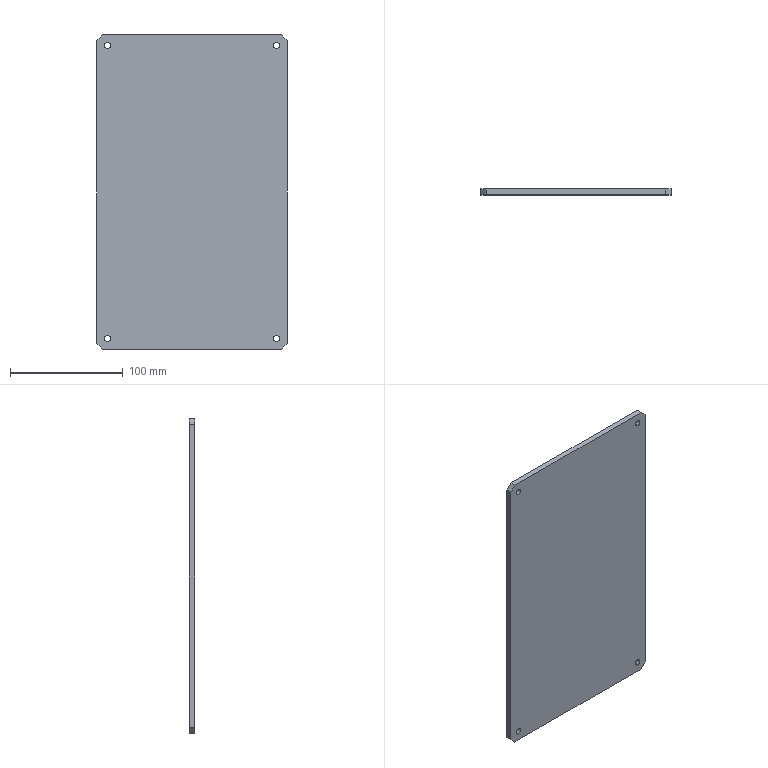Part | SolidWorks | features Chamfer 1, Extrusion 1, HoleWzd 1 | 1 solid | 18 faces | box 169 x 5 x 279 mm | volume 235030 mm3 | plane 10 | cylinder 8 | commonest cylinder face diameters 5.5 x8
STEP:
#1=CARTESIAN_POINT('',(-75.,2.5,132.75));
#2=VERTEX_POINT('',#1);
#3=CARTESIAN_POINT('',(-75.,2.5,127.25));
#4=VERTEX_POINT('',#3);
#5=CARTESIAN_POINT('',(-75.,2.5,130.));
#6=DIRECTION('',(0.,-1.,0.));
#7=DIRECTION('',(0.,0.,-1.));
#8=AXIS2_PLACEMENT_3D('',#5,#6,#7);
#9=CIRCLE('',#8,2.75);
#10=EDGE_CURVE('',#2,#4,#9,.T.);
#11=ORIENTED_EDGE('',*,*,#10,.F.);
#12=CARTESIAN_POINT('',(-75.,-2.5,132.75));
#13=VERTEX_POINT('',#12);
#14=CARTESIAN_POINT('',(-75.,-2.5,132.75));
#15=DIRECTION('',(0.,-1.,0.));
#16=VECTOR('',#15,1000.);
#17=LINE('',#14,#16);
#18=EDGE_CURVE('',#2,#13,#17,.T.);
#19=ORIENTED_EDGE('',*,*,#18,.T.);
#20=CARTESIAN_POINT('',(-75.,-2.5,127.25));
#21=VERTEX_POINT('',#20);
#22=CARTESIAN_POINT('',(-75.,-2.5,130.));
#23=DIRECTION('',(0.,-1.,0.));
#24=DIRECTION('',(0.,0.,-1.));
#25=AXIS2_PLACEMENT_3D('',#22,#23,#24);
#26=CIRCLE('',#25,2.75);
#27=EDGE_CURVE('',#13,#21,#26,.T.);
#28=ORIENTED_EDGE('',*,*,#27,.T.);
#29=CARTESIAN_POINT('',(-75.,-2.5,127.25));
#30=DIRECTION('',(0.,-1.,0.));
#31=VECTOR('',#30,1000.);
#32=LINE('',#29,#31);
#33=EDGE_CURVE('',#4,#21,#32,.T.);
#34=ORIENTED_EDGE('',*,*,#33,.F.);
#35=EDGE_LOOP('',(#11,#19,#28,#34));
#36=FACE_OUTER_BOUND('',#35,.T.);
#37=CARTESIAN_POINT('',(-75.,-2.5,130.));
#38=DIRECTION('',(0.,-1.,0.));
#39=DIRECTION('',(0.,0.,-1.));
#40=AXIS2_PLACEMENT_3D('',#37,#38,#39);
#41=CYLINDRICAL_SURFACE('',#40,2.75);
#42=ADVANCED_FACE('',(#36),#41,.F.);
#43=CARTESIAN_POINT('',(75.,2.5,132.75));
#44=VERTEX_POINT('',#43);
#45=CARTESIAN_POINT('',(75.,2.5,127.25));
#46=VERTEX_POINT('',#45);
#47=CARTESIAN_POINT('',(75.,2.5,130.));
#48=DIRECTION('',(0.,-1.,0.));
#49=DIRECTION('',(0.,0.,-1.));
#50=AXIS2_PLACEMENT_3D('',#47,#48,#49);
#51=CIRCLE('',#50,2.75);
#52=EDGE_CURVE('',#44,#46,#51,.T.);
#53=ORIENTED_EDGE('',*,*,#52,.F.);
#54=CARTESIAN_POINT('',(75.,-2.5,132.75));
#55=VERTEX_POINT('',#54);
#56=CARTESIAN_POINT('',(75.,-2.5,132.75));
#57=DIRECTION('',(0.,-1.,0.));
#58=VECTOR('',#57,1000.);
#59=LINE('',#56,#58);
#60=EDGE_CURVE('',#44,#55,#59,.T.);
#61=ORIENTED_EDGE('',*,*,#60,.T.);
#62=CARTESIAN_POINT('',(75.,-2.5,127.25));
#63=VERTEX_POINT('',#62);
#64=CARTESIAN_POINT('',(75.,-2.5,130.));
#65=DIRECTION('',(0.,-1.,0.));
#66=DIRECTION('',(0.,0.,-1.));
#67=AXIS2_PLACEMENT_3D('',#64,#65,#66);
#68=CIRCLE('',#67,2.75);
#69=EDGE_CURVE('',#55,#63,#68,.T.);
#70=ORIENTED_EDGE('',*,*,#69,.T.);
#71=CARTESIAN_POINT('',(75.,-2.5,127.25));
#72=DIRECTION('',(0.,-1.,0.));
#73=VECTOR('',#72,1000.);
#74=LINE('',#71,#73);
#75=EDGE_CURVE('',#46,#63,#74,.T.);
#76=ORIENTED_EDGE('',*,*,#75,.F.);
#77=EDGE_LOOP('',(#53,#61,#70,#76));
#78=FACE_OUTER_BOUND('',#77,.T.);
#79=CARTESIAN_POINT('',(75.,-2.5,130.));
#80=DIRECTION('',(0.,-1.,0.));
#81=DIRECTION('',(0.,0.,-1.));
#82=AXIS2_PLACEMENT_3D('',#79,#80,#81);
#83=CYLINDRICAL_SURFACE('',#82,2.75);
#84=ADVANCED_FACE('',(#78),#83,.F.);
#85=CARTESIAN_POINT('',(75.,2.5,-127.25));
#86=VERTEX_POINT('',#85);
#87=CARTESIAN_POINT('',(75.,2.5,-132.75));
#88=VERTEX_POINT('',#87);
#89=CARTESIAN_POINT('',(75.,2.5,-130.));
#90=DIRECTION('',(0.,-1.,0.));
#91=DIRECTION('',(0.,0.,-1.));
#92=AXIS2_PLACEMENT_3D('',#89,#90,#91);
#93=CIRCLE('',#92,2.75);
#94=EDGE_CURVE('',#86,#88,#93,.T.);
#95=ORIENTED_EDGE('',*,*,#94,.F.);
#96=CARTESIAN_POINT('',(75.,-2.5,-127.25));
#97=VERTEX_POINT('',#96);
#98=CARTESIAN_POINT('',(75.,-2.5,-127.25));
#99=DIRECTION('',(0.,-1.,0.));
#100=VECTOR('',#99,1000.);
#101=LINE('',#98,#100);
#102=EDGE_CURVE('',#86,#97,#101,.T.);
#103=ORIENTED_EDGE('',*,*,#102,.T.);
#104=CARTESIAN_POINT('',(75.,-2.5,-132.75));
#105=VERTEX_POINT('',#104);
#106=CARTESIAN_POINT('',(75.,-2.5,-130.));
#107=DIRECTION('',(0.,-1.,0.));
#108=DIRECTION('',(0.,0.,-1.));
#109=AXIS2_PLACEMENT_3D('',#106,#107,#108);
#110=CIRCLE('',#109,2.75);
#111=EDGE_CURVE('',#97,#105,#110,.T.);
#112=ORIENTED_EDGE('',*,*,#111,.T.);
#113=CARTESIAN_POINT('',(75.,-2.5,-132.75));
#114=DIRECTION('',(0.,-1.,0.));
#115=VECTOR('',#114,1000.);
#116=LINE('',#113,#115);
#117=EDGE_CURVE('',#88,#105,#116,.T.);
#118=ORIENTED_EDGE('',*,*,#117,.F.);
#119=EDGE_LOOP('',(#95,#103,#112,#118));
#120=FACE_OUTER_BOUND('',#119,.T.);
#121=CARTESIAN_POINT('',(75.,-2.5,-130.));
#122=DIRECTION('',(0.,-1.,0.));
#123=DIRECTION('',(0.,0.,-1.));
#124=AXIS2_PLACEMENT_3D('',#121,#122,#123);
#125=CYLINDRICAL_SURFACE('',#124,2.75);
#126=ADVANCED_FACE('',(#120),#125,.F.);
#127=CARTESIAN_POINT('',(-75.,2.5,-127.25));
#128=VERTEX_POINT('',#127);
#129=CARTESIAN_POINT('',(-75.,2.5,-132.75));
#130=VERTEX_POINT('',#129);
#131=CARTESIAN_POINT('',(-75.,2.5,-130.));
#132=DIRECTION('',(0.,-1.,0.));
#133=DIRECTION('',(0.,0.,-1.));
#134=AXIS2_PLACEMENT_3D('',#131,#132,#133);
#135=CIRCLE('',#134,2.75);
#136=EDGE_CURVE('',#128,#130,#135,.T.);
#137=ORIENTED_EDGE('',*,*,#136,.F.);
#138=CARTESIAN_POINT('',(-75.,-2.5,-127.25));
#139=VERTEX_POINT('',#138);
#140=CARTESIAN_POINT('',(-75.,-2.5,-127.25));
#141=DIRECTION('',(0.,-1.,0.));
#142=VECTOR('',#141,1000.);
#143=LINE('',#140,#142);
#144=EDGE_CURVE('',#128,#139,#143,.T.);
#145=ORIENTED_EDGE('',*,*,#144,.T.);
#146=CARTESIAN_POINT('',(-75.,-2.5,-132.75));
#147=VERTEX_POINT('',#146);
#148=CARTESIAN_POINT('',(-75.,-2.5,-130.));
#149=DIRECTION('',(0.,-1.,0.));
#150=DIRECTION('',(0.,0.,-1.));
#151=AXIS2_PLACEMENT_3D('',#148,#149,#150);
#152=CIRCLE('',#151,2.75);
#153=EDGE_CURVE('',#139,#147,#152,.T.);
#154=ORIENTED_EDGE('',*,*,#153,.T.);
#155=CARTESIAN_POINT('',(-75.,-2.5,-132.75));
#156=DIRECTION('',(0.,-1.,0.));
#157=VECTOR('',#156,1000.);
#158=LINE('',#155,#157);
#159=EDGE_CURVE('',#130,#147,#158,.T.);
#160=ORIENTED_EDGE('',*,*,#159,.F.);
#161=EDGE_LOOP('',(#137,#145,#154,#160));
#162=FACE_OUTER_BOUND('',#161,.T.);
#163=CARTESIAN_POINT('',(-75.,-2.5,-130.));
#164=DIRECTION('',(0.,-1.,0.));
#165=DIRECTION('',(0.,0.,-1.));
#166=AXIS2_PLACEMENT_3D('',#163,#164,#165);
#167=CYLINDRICAL_SURFACE('',#166,2.75);
#168=ADVANCED_FACE('',(#162),#167,.F.);
#169=CARTESIAN_POINT('',(-84.5,2.5,-134.5));
#170=VERTEX_POINT('',#169);
#171=CARTESIAN_POINT('',(-84.5,2.5,134.5));
#172=VERTEX_POINT('',#171);
#173=CARTESIAN_POINT('',(-84.5,2.5,139.5));
#174=DIRECTION('',(0.,0.,1.));
#175=VECTOR('',#174,1000.);
#176=LINE('',#173,#175);
#177=EDGE_CURVE('',#170,#172,#176,.T.);
#178=ORIENTED_EDGE('',*,*,#177,.F.);
#179=CARTESIAN_POINT('',(-84.5,-2.5,-134.5));
#180=VERTEX_POINT('',#179);
#181=CARTESIAN_POINT('',(-84.5,2.5,-134.5));
#182=DIRECTION('',(0.,-1.,0.));
#183=VECTOR('',#182,1000.);
#184=LINE('',#181,#183);
#185=EDGE_CURVE('',#170,#180,#184,.T.);
#186=ORIENTED_EDGE('',*,*,#185,.T.);
#187=CARTESIAN_POINT('',(-84.5,-2.5,134.5));
#188=VERTEX_POINT('',#187);
#189=CARTESIAN_POINT('',(-84.5,-2.5,139.5));
#190=DIRECTION('',(0.,0.,1.));
#191=VECTOR('',#190,1000.);
#192=LINE('',#189,#191);
#193=EDGE_CURVE('',#180,#188,#192,.T.);
#194=ORIENTED_EDGE('',*,*,#193,.T.);
#195=CARTESIAN_POINT('',(-84.5,2.5,134.5));
#196=DIRECTION('',(0.,1.,0.));
#197=VECTOR('',#196,1000.);
#198=LINE('',#195,#197);
#199=EDGE_CURVE('',#188,#172,#198,.T.);
#200=ORIENTED_EDGE('',*,*,#199,.T.);
#201=EDGE_LOOP('',(#178,#186,#194,#200));
#202=FACE_OUTER_BOUND('',#201,.T.);
#203=CARTESIAN_POINT('',(-84.5,2.5,139.5));
#204=DIRECTION('',(1.,0.,0.));
#205=DIRECTION('',(0.,0.,-1.));
#206=AXIS2_PLACEMENT_3D('',#203,#204,#205);
#207=PLANE('',#206);
#208=ADVANCED_FACE('',(#202),#207,.F.);
#209=CARTESIAN_POINT('',(-79.5,-2.5,139.5));
#210=VERTEX_POINT('',#209);
#211=CARTESIAN_POINT('',(79.5,-2.5,139.5));
#212=VERTEX_POINT('',#211);
#213=CARTESIAN_POINT('',(84.5,-2.5,139.5));
#214=DIRECTION('',(1.,0.,0.));
#215=VECTOR('',#214,1000.);
#216=LINE('',#213,#215);
#217=EDGE_CURVE('',#210,#212,#216,.T.);
#218=ORIENTED_EDGE('',*,*,#217,.T.);
#219=CARTESIAN_POINT('',(79.5,2.5,139.5));
#220=VERTEX_POINT('',#219);
#221=CARTESIAN_POINT('',(79.5,2.5,139.5));
#222=DIRECTION('',(0.,1.,0.));
#223=VECTOR('',#222,1000.);
#224=LINE('',#221,#223);
#225=EDGE_CURVE('',#212,#220,#224,.T.);
#226=ORIENTED_EDGE('',*,*,#225,.T.);
#227=CARTESIAN_POINT('',(-79.5,2.5,139.5));
#228=VERTEX_POINT('',#227);
#229=CARTESIAN_POINT('',(84.5,2.5,139.5));
#230=DIRECTION('',(1.,0.,0.));
#231=VECTOR('',#230,1000.);
#232=LINE('',#229,#231);
#233=EDGE_CURVE('',#228,#220,#232,.T.);
#234=ORIENTED_EDGE('',*,*,#233,.F.);
#235=CARTESIAN_POINT('',(-79.5,2.5,139.5));
#236=DIRECTION('',(0.,-1.,0.));
#237=VECTOR('',#236,1000.);
#238=LINE('',#235,#237);
#239=EDGE_CURVE('',#228,#210,#238,.T.);
#240=ORIENTED_EDGE('',*,*,#239,.T.);
#241=EDGE_LOOP('',(#218,#226,#234,#240));
#242=FACE_OUTER_BOUND('',#241,.T.);
#243=CARTESIAN_POINT('',(84.5,2.5,139.5));
#244=DIRECTION('',(0.,0.,-1.));
#245=DIRECTION('',(-1.,0.,0.));
#246=AXIS2_PLACEMENT_3D('',#243,#244,#245);
#247=PLANE('',#246);
#248=ADVANCED_FACE('',(#242),#247,.F.);
#249=CARTESIAN_POINT('',(84.5,-2.5,134.5));
#250=VERTEX_POINT('',#249);
#251=CARTESIAN_POINT('',(84.5,-2.5,-134.5));
#252=VERTEX_POINT('',#251);
#253=CARTESIAN_POINT('',(84.5,-2.5,139.5));
#254=DIRECTION('',(0.,0.,-1.));
#255=VECTOR('',#254,1000.);
#256=LINE('',#253,#255);
#257=EDGE_CURVE('',#250,#252,#256,.T.);
#258=ORIENTED_EDGE('',*,*,#257,.T.);
#259=CARTESIAN_POINT('',(84.5,2.5,-134.5));
#260=VERTEX_POINT('',#259);
#261=CARTESIAN_POINT('',(84.5,2.5,-134.5));
#262=DIRECTION('',(0.,1.,0.));
#263=VECTOR('',#262,1000.);
#264=LINE('',#261,#263);
#265=EDGE_CURVE('',#252,#260,#264,.T.);
#266=ORIENTED_EDGE('',*,*,#265,.T.);
#267=CARTESIAN_POINT('',(84.5,2.5,134.5));
#268=VERTEX_POINT('',#267);
#269=CARTESIAN_POINT('',(84.5,2.5,139.5));
#270=DIRECTION('',(0.,0.,-1.));
#271=VECTOR('',#270,1000.);
#272=LINE('',#269,#271);
#273=EDGE_CURVE('',#268,#260,#272,.T.);
#274=ORIENTED_EDGE('',*,*,#273,.F.);
#275=CARTESIAN_POINT('',(84.5,2.5,134.5));
#276=DIRECTION('',(0.,-1.,0.));
#277=VECTOR('',#276,1000.);
#278=LINE('',#275,#277);
#279=EDGE_CURVE('',#268,#250,#278,.T.);
#280=ORIENTED_EDGE('',*,*,#279,.T.);
#281=EDGE_LOOP('',(#258,#266,#274,#280));
#282=FACE_OUTER_BOUND('',#281,.T.);
#283=CARTESIAN_POINT('',(84.5,2.5,139.5));
#284=DIRECTION('',(-1.,0.,0.));
#285=DIRECTION('',(0.,0.,1.));
#286=AXIS2_PLACEMENT_3D('',#283,#284,#285);
#287=PLANE('',#286);
#288=ADVANCED_FACE('',(#282),#287,.F.);
#289=CARTESIAN_POINT('',(79.5,2.5,-139.5));
#290=VERTEX_POINT('',#289);
#291=CARTESIAN_POINT('',(-79.5,2.5,-139.5));
#292=VERTEX_POINT('',#291);
#293=CARTESIAN_POINT('',(84.5,2.5,-139.5));
#294=DIRECTION('',(-1.,0.,0.));
#295=VECTOR('',#294,1000.);
#296=LINE('',#293,#295);
#297=EDGE_CURVE('',#290,#292,#296,.T.);
#298=ORIENTED_EDGE('',*,*,#297,.F.);
#299=CARTESIAN_POINT('',(79.5,-2.5,-139.5));
#300=VERTEX_POINT('',#299);
#301=CARTESIAN_POINT('',(79.5,2.5,-139.5));
#302=DIRECTION('',(0.,-1.,0.));
#303=VECTOR('',#302,1000.);
#304=LINE('',#301,#303);
#305=EDGE_CURVE('',#290,#300,#304,.T.);
#306=ORIENTED_EDGE('',*,*,#305,.T.);
#307=CARTESIAN_POINT('',(-79.5,-2.5,-139.5));
#308=VERTEX_POINT('',#307);
#309=CARTESIAN_POINT('',(84.5,-2.5,-139.5));
#310=DIRECTION('',(-1.,0.,0.));
#311=VECTOR('',#310,1000.);
#312=LINE('',#309,#311);
#313=EDGE_CURVE('',#300,#308,#312,.T.);
#314=ORIENTED_EDGE('',*,*,#313,.T.);
#315=CARTESIAN_POINT('',(-79.5,2.5,-139.5));
#316=DIRECTION('',(0.,1.,0.));
#317=VECTOR('',#316,1000.);
#318=LINE('',#315,#317);
#319=EDGE_CURVE('',#308,#292,#318,.T.);
#320=ORIENTED_EDGE('',*,*,#319,.T.);
#321=EDGE_LOOP('',(#298,#306,#314,#320));
#322=FACE_OUTER_BOUND('',#321,.T.);
#323=CARTESIAN_POINT('',(84.5,2.5,-139.5));
#324=DIRECTION('',(0.,0.,1.));
#325=DIRECTION('',(1.,0.,0.));
#326=AXIS2_PLACEMENT_3D('',#323,#324,#325);
#327=PLANE('',#326);
#328=ADVANCED_FACE('',(#322),#327,.F.);
#329=CARTESIAN_POINT('',(-75.,2.5,130.));
#330=DIRECTION('',(0.,-1.,0.));
#331=DIRECTION('',(0.,0.,-1.));
#332=AXIS2_PLACEMENT_3D('',#329,#330,#331);
#333=CIRCLE('',#332,2.75);
#334=EDGE_CURVE('',#4,#2,#333,.T.);
#335=ORIENTED_EDGE('',*,*,#334,.T.);
#336=ORIENTED_EDGE('',*,*,#10,.T.);
#337=EDGE_LOOP('',(#335,#336));
#338=FACE_BOUND('',#337,.T.);
#339=CARTESIAN_POINT('',(75.,2.5,130.));
#340=DIRECTION('',(0.,-1.,0.));
#341=DIRECTION('',(0.,0.,-1.));
#342=AXIS2_PLACEMENT_3D('',#339,#340,#341);
#343=CIRCLE('',#342,2.75);
#344=EDGE_CURVE('',#46,#44,#343,.T.);
#345=ORIENTED_EDGE('',*,*,#344,.T.);
#346=ORIENTED_EDGE('',*,*,#52,.T.);
#347=EDGE_LOOP('',(#345,#346));
#348=FACE_BOUND('',#347,.T.);
#349=CARTESIAN_POINT('',(75.,2.5,-130.));
#350=DIRECTION('',(0.,-1.,0.));
#351=DIRECTION('',(0.,0.,-1.));
#352=AXIS2_PLACEMENT_3D('',#349,#350,#351);
#353=CIRCLE('',#352,2.75);
#354=EDGE_CURVE('',#88,#86,#353,.T.);
#355=ORIENTED_EDGE('',*,*,#354,.T.);
#356=ORIENTED_EDGE('',*,*,#94,.T.);
#357=EDGE_LOOP('',(#355,#356));
#358=FACE_BOUND('',#357,.T.);
#359=CARTESIAN_POINT('',(-75.,2.5,-130.));
#360=DIRECTION('',(0.,-1.,0.));
#361=DIRECTION('',(0.,0.,-1.));
#362=AXIS2_PLACEMENT_3D('',#359,#360,#361);
#363=CIRCLE('',#362,2.75);
#364=EDGE_CURVE('',#130,#128,#363,.T.);
#365=ORIENTED_EDGE('',*,*,#364,.T.);
#366=ORIENTED_EDGE('',*,*,#136,.T.);
#367=EDGE_LOOP('',(#365,#366));
#368=FACE_BOUND('',#367,.T.);
#369=ORIENTED_EDGE('',*,*,#273,.T.);
#370=CARTESIAN_POINT('',(109.5,2.5,-109.5));
#371=DIRECTION('',(-0.7071,0.,-0.7071));
#372=VECTOR('',#371,1000.);
#373=LINE('',#370,#372);
#374=EDGE_CURVE('',#260,#290,#373,.T.);
#375=ORIENTED_EDGE('',*,*,#374,.T.);
#376=ORIENTED_EDGE('',*,*,#297,.T.);
#377=CARTESIAN_POINT('',(-109.5,2.5,-109.5));
#378=DIRECTION('',(-0.7071,0.,0.7071));
#379=VECTOR('',#378,1000.);
#380=LINE('',#377,#379);
#381=EDGE_CURVE('',#292,#170,#380,.T.);
#382=ORIENTED_EDGE('',*,*,#381,.T.);
#383=ORIENTED_EDGE('',*,*,#177,.T.);
#384=CARTESIAN_POINT('',(-109.5,2.5,109.5));
#385=DIRECTION('',(0.7071,0.,0.7071));
#386=VECTOR('',#385,1000.);
#387=LINE('',#384,#386);
#388=EDGE_CURVE('',#172,#228,#387,.T.);
#389=ORIENTED_EDGE('',*,*,#388,.T.);
#390=ORIENTED_EDGE('',*,*,#233,.T.);
#391=CARTESIAN_POINT('',(109.5,2.5,109.5));
#392=DIRECTION('',(0.7071,0.,-0.7071));
#393=VECTOR('',#392,1000.);
#394=LINE('',#391,#393);
#395=EDGE_CURVE('',#220,#268,#394,.T.);
#396=ORIENTED_EDGE('',*,*,#395,.T.);
#397=EDGE_LOOP('',(#369,#375,#376,#382,#383,#389,#390,#396));
#398=FACE_OUTER_BOUND('',#397,.T.);
#399=CARTESIAN_POINT('',(0.,2.5,0.));
#400=DIRECTION('',(0.,1.,0.));
#401=DIRECTION('',(0.,0.,1.));
#402=AXIS2_PLACEMENT_3D('',#399,#400,#401);
#403=PLANE('',#402);
#404=ADVANCED_FACE('',(#338,#348,#358,#368,#398),#403,.T.);
#405=CARTESIAN_POINT('',(-75.,-2.5,130.));
#406=DIRECTION('',(0.,-1.,0.));
#407=DIRECTION('',(0.,0.,-1.));
#408=AXIS2_PLACEMENT_3D('',#405,#406,#407);
#409=CIRCLE('',#408,2.75);
#410=EDGE_CURVE('',#21,#13,#409,.T.);
#411=ORIENTED_EDGE('',*,*,#410,.F.);
#412=ORIENTED_EDGE('',*,*,#27,.F.);
#413=EDGE_LOOP('',(#411,#412));
#414=FACE_BOUND('',#413,.T.);
#415=CARTESIAN_POINT('',(75.,-2.5,130.));
#416=DIRECTION('',(0.,-1.,0.));
#417=DIRECTION('',(0.,0.,-1.));
#418=AXIS2_PLACEMENT_3D('',#415,#416,#417);
#419=CIRCLE('',#418,2.75);
#420=EDGE_CURVE('',#63,#55,#419,.T.);
#421=ORIENTED_EDGE('',*,*,#420,.F.);
#422=ORIENTED_EDGE('',*,*,#69,.F.);
#423=EDGE_LOOP('',(#421,#422));
#424=FACE_BOUND('',#423,.T.);
#425=CARTESIAN_POINT('',(75.,-2.5,-130.));
#426=DIRECTION('',(0.,-1.,0.));
#427=DIRECTION('',(0.,0.,-1.));
#428=AXIS2_PLACEMENT_3D('',#425,#426,#427);
#429=CIRCLE('',#428,2.75);
#430=EDGE_CURVE('',#105,#97,#429,.T.);
#431=ORIENTED_EDGE('',*,*,#430,.F.);
#432=ORIENTED_EDGE('',*,*,#111,.F.);
#433=EDGE_LOOP('',(#431,#432));
#434=FACE_BOUND('',#433,.T.);
#435=CARTESIAN_POINT('',(-75.,-2.5,-130.));
#436=DIRECTION('',(0.,-1.,0.));
#437=DIRECTION('',(0.,0.,-1.));
#438=AXIS2_PLACEMENT_3D('',#435,#436,#437);
#439=CIRCLE('',#438,2.75);
#440=EDGE_CURVE('',#147,#139,#439,.T.);
#441=ORIENTED_EDGE('',*,*,#440,.F.);
#442=ORIENTED_EDGE('',*,*,#153,.F.);
#443=EDGE_LOOP('',(#441,#442));
#444=FACE_BOUND('',#443,.T.);
#445=ORIENTED_EDGE('',*,*,#313,.F.);
#446=CARTESIAN_POINT('',(79.5,-2.5,-139.5));
#447=DIRECTION('',(0.7071,0.,0.7071));
#448=VECTOR('',#447,1000.);
#449=LINE('',#446,#448);
#450=EDGE_CURVE('',#300,#252,#449,.T.);
#451=ORIENTED_EDGE('',*,*,#450,.T.);
#452=ORIENTED_EDGE('',*,*,#257,.F.);
#453=CARTESIAN_POINT('',(84.5,-2.5,134.5));
#454=DIRECTION('',(-0.7071,0.,0.7071));
#455=VECTOR('',#454,1000.);
#456=LINE('',#453,#455);
#457=EDGE_CURVE('',#250,#212,#456,.T.);
#458=ORIENTED_EDGE('',*,*,#457,.T.);
#459=ORIENTED_EDGE('',*,*,#217,.F.);
#460=CARTESIAN_POINT('',(-79.5,-2.5,139.5));
#461=DIRECTION('',(-0.7071,0.,-0.7071));
#462=VECTOR('',#461,1000.);
#463=LINE('',#460,#462);
#464=EDGE_CURVE('',#210,#188,#463,.T.);
#465=ORIENTED_EDGE('',*,*,#464,.T.);
#466=ORIENTED_EDGE('',*,*,#193,.F.);
#467=CARTESIAN_POINT('',(-84.5,-2.5,-134.5));
#468=DIRECTION('',(0.7071,0.,-0.7071));
#469=VECTOR('',#468,1000.);
#470=LINE('',#467,#469);
#471=EDGE_CURVE('',#180,#308,#470,.T.);
#472=ORIENTED_EDGE('',*,*,#471,.T.);
#473=EDGE_LOOP('',(#445,#451,#452,#458,#459,#465,#466,#472));
#474=FACE_OUTER_BOUND('',#473,.T.);
#475=CARTESIAN_POINT('',(0.,-2.5,0.));
#476=DIRECTION('',(0.,1.,0.));
#477=DIRECTION('',(0.,0.,1.));
#478=AXIS2_PLACEMENT_3D('',#475,#476,#477);
#479=PLANE('',#478);
#480=ADVANCED_FACE('',(#414,#424,#434,#444,#474),#479,.F.);
#481=ORIENTED_EDGE('',*,*,#144,.F.);
#482=ORIENTED_EDGE('',*,*,#364,.F.);
#483=ORIENTED_EDGE('',*,*,#159,.T.);
#484=ORIENTED_EDGE('',*,*,#440,.T.);
#485=EDGE_LOOP('',(#481,#482,#483,#484));
#486=FACE_OUTER_BOUND('',#485,.T.);
#487=CARTESIAN_POINT('',(-75.,-2.5,-130.));
#488=DIRECTION('',(0.,-1.,0.));
#489=DIRECTION('',(0.,0.,-1.));
#490=AXIS2_PLACEMENT_3D('',#487,#488,#489);
#491=CYLINDRICAL_SURFACE('',#490,2.75);
#492=ADVANCED_FACE('',(#486),#491,.F.);
#493=ORIENTED_EDGE('',*,*,#102,.F.);
#494=ORIENTED_EDGE('',*,*,#354,.F.);
#495=ORIENTED_EDGE('',*,*,#117,.T.);
#496=ORIENTED_EDGE('',*,*,#430,.T.);
#497=EDGE_LOOP('',(#493,#494,#495,#496));
#498=FACE_OUTER_BOUND('',#497,.T.);
#499=CARTESIAN_POINT('',(75.,-2.5,-130.));
#500=DIRECTION('',(0.,-1.,0.));
#501=DIRECTION('',(0.,0.,-1.));
#502=AXIS2_PLACEMENT_3D('',#499,#500,#501);
#503=CYLINDRICAL_SURFACE('',#502,2.75);
#504=ADVANCED_FACE('',(#498),#503,.F.);
#505=ORIENTED_EDGE('',*,*,#60,.F.);
#506=ORIENTED_EDGE('',*,*,#344,.F.);
#507=ORIENTED_EDGE('',*,*,#75,.T.);
#508=ORIENTED_EDGE('',*,*,#420,.T.);
#509=EDGE_LOOP('',(#505,#506,#507,#508));
#510=FACE_OUTER_BOUND('',#509,.T.);
#511=CARTESIAN_POINT('',(75.,-2.5,130.));
#512=DIRECTION('',(0.,-1.,0.));
#513=DIRECTION('',(0.,0.,-1.));
#514=AXIS2_PLACEMENT_3D('',#511,#512,#513);
#515=CYLINDRICAL_SURFACE('',#514,2.75);
#516=ADVANCED_FACE('',(#510),#515,.F.);
#517=ORIENTED_EDGE('',*,*,#18,.F.);
#518=ORIENTED_EDGE('',*,*,#334,.F.);
#519=ORIENTED_EDGE('',*,*,#33,.T.);
#520=ORIENTED_EDGE('',*,*,#410,.T.);
#521=EDGE_LOOP('',(#517,#518,#519,#520));
#522=FACE_OUTER_BOUND('',#521,.T.);
#523=CARTESIAN_POINT('',(-75.,-2.5,130.));
#524=DIRECTION('',(0.,-1.,0.));
#525=DIRECTION('',(0.,0.,-1.));
#526=AXIS2_PLACEMENT_3D('',#523,#524,#525);
#527=CYLINDRICAL_SURFACE('',#526,2.75);
#528=ADVANCED_FACE('',(#522),#527,.F.);
#529=ORIENTED_EDGE('',*,*,#374,.F.);
#530=ORIENTED_EDGE('',*,*,#265,.F.);
#531=ORIENTED_EDGE('',*,*,#450,.F.);
#532=ORIENTED_EDGE('',*,*,#305,.F.);
#533=EDGE_LOOP('',(#529,#530,#531,#532));
#534=FACE_OUTER_BOUND('',#533,.T.);
#535=CARTESIAN_POINT('',(79.5,2.5,-139.5));
#536=DIRECTION('',(-0.7071,0.,0.7071));
#537=DIRECTION('',(0.,-1.,0.));
#538=AXIS2_PLACEMENT_3D('',#535,#536,#537);
#539=PLANE('',#538);
#540=ADVANCED_FACE('',(#534),#539,.F.);
#541=ORIENTED_EDGE('',*,*,#381,.F.);
#542=ORIENTED_EDGE('',*,*,#319,.F.);
#543=ORIENTED_EDGE('',*,*,#471,.F.);
#544=ORIENTED_EDGE('',*,*,#185,.F.);
#545=EDGE_LOOP('',(#541,#542,#543,#544));
#546=FACE_OUTER_BOUND('',#545,.T.);
#547=CARTESIAN_POINT('',(-84.5,2.5,-134.5));
#548=DIRECTION('',(0.7071,0.,0.7071));
#549=DIRECTION('',(0.,-1.,0.));
#550=AXIS2_PLACEMENT_3D('',#547,#548,#549);
#551=PLANE('',#550);
#552=ADVANCED_FACE('',(#546),#551,.F.);
#553=ORIENTED_EDGE('',*,*,#395,.F.);
#554=ORIENTED_EDGE('',*,*,#225,.F.);
#555=ORIENTED_EDGE('',*,*,#457,.F.);
#556=ORIENTED_EDGE('',*,*,#279,.F.);
#557=EDGE_LOOP('',(#553,#554,#555,#556));
#558=FACE_OUTER_BOUND('',#557,.T.);
#559=CARTESIAN_POINT('',(84.5,2.5,134.5));
#560=DIRECTION('',(-0.7071,0.,-0.7071));
#561=DIRECTION('',(0.,-1.,0.));
#562=AXIS2_PLACEMENT_3D('',#559,#560,#561);
#563=PLANE('',#562);
#564=ADVANCED_FACE('',(#558),#563,.F.);
#565=ORIENTED_EDGE('',*,*,#388,.F.);
#566=ORIENTED_EDGE('',*,*,#199,.F.);
#567=ORIENTED_EDGE('',*,*,#464,.F.);
#568=ORIENTED_EDGE('',*,*,#239,.F.);
#569=EDGE_LOOP('',(#565,#566,#567,#568));
#570=FACE_OUTER_BOUND('',#569,.T.);
#571=CARTESIAN_POINT('',(-79.5,2.5,139.5));
#572=DIRECTION('',(0.7071,0.,-0.7071));
#573=DIRECTION('',(0.,-1.,0.));
#574=AXIS2_PLACEMENT_3D('',#571,#572,#573);
#575=PLANE('',#574);
#576=ADVANCED_FACE('',(#570),#575,.F.);
#577=CLOSED_SHELL('',(#42,#84,#126,#168,#208,#248,#288,#328,#404,#480,#492,#504,#516,#528,#540,#552,#564,#576));
#578=MANIFOLD_SOLID_BREP('',#577);
#579=CARTESIAN_POINT('',(0.,0.,0.));
#580=DIRECTION('',(0.,0.,1.));
#581=DIRECTION('',(1.,0.,0.));
#582=AXIS2_PLACEMENT_3D('',#579,#580,#581);
#583=(LENGTH_UNIT()NAMED_UNIT(*)SI_UNIT(.MILLI.,.METRE.));
#584=UNCERTAINTY_MEASURE_WITH_UNIT(LENGTH_MEASURE(0.00001),#583,'','');
#585=(NAMED_UNIT(*)PLANE_ANGLE_UNIT()SI_UNIT($,.RADIAN.));
#586=(NAMED_UNIT(*)SI_UNIT($,.STERADIAN.)SOLID_ANGLE_UNIT());
#587=(GEOMETRIC_REPRESENTATION_CONTEXT(3)GLOBAL_UNCERTAINTY_ASSIGNED_CONTEXT((#584))GLOBAL_UNIT_ASSIGNED_CONTEXT((#583,#585,#586))REPRESENTATION_CONTEXT('',''));
#588=ADVANCED_BREP_SHAPE_REPRESENTATION('',(#578,#582),#587);